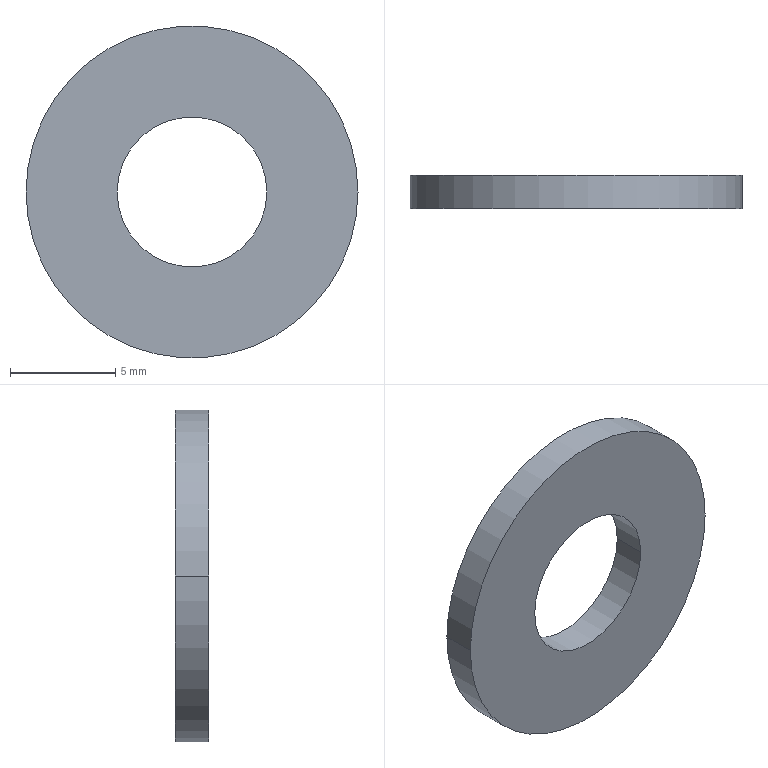Part | NX | features BREP 1 | 1 solid | 6 faces | box 15.748 x 1.575 x 15.748 mm | volume 244.177 mm3 | cylinder 4 | plane 2 | commonest cylinder face diameters 7.112 x2 15.748 x2
STEP:
#1=CARTESIAN_POINT('',(-7.874,0.,0.));
#2=VERTEX_POINT('',#1);
#3=CARTESIAN_POINT('',(7.874,0.,0.));
#4=VERTEX_POINT('',#3);
#5=CARTESIAN_POINT('',(0.,0.,0.));
#6=DIRECTION('',(0.,1.,0.));
#7=DIRECTION('',(-1.,0.,0.));
#8=AXIS2_PLACEMENT_3D('',#5,#6,#7);
#9=CIRCLE('',#8,7.874);
#10=EDGE_CURVE('',#2,#4,#9,.T.);
#11=ORIENTED_EDGE('',*,*,#10,.F.);
#12=CARTESIAN_POINT('',(0.,0.,0.));
#13=DIRECTION('',(0.,1.,0.));
#14=DIRECTION('',(1.,0.,0.));
#15=AXIS2_PLACEMENT_3D('',#12,#13,#14);
#16=CIRCLE('',#15,7.874);
#17=EDGE_CURVE('',#4,#2,#16,.T.);
#18=ORIENTED_EDGE('',*,*,#17,.F.);
#19=EDGE_LOOP('',(#11,#18));
#20=FACE_BOUND('',#19,.T.);
#21=CARTESIAN_POINT('',(-3.556,0.,0.));
#22=VERTEX_POINT('',#21);
#23=CARTESIAN_POINT('',(3.556,0.,0.));
#24=VERTEX_POINT('',#23);
#25=CARTESIAN_POINT('',(0.,0.,0.));
#26=DIRECTION('',(0.,-1.,0.));
#27=DIRECTION('',(-1.,0.,0.));
#28=AXIS2_PLACEMENT_3D('',#25,#26,#27);
#29=CIRCLE('',#28,3.556);
#30=EDGE_CURVE('',#22,#24,#29,.T.);
#31=ORIENTED_EDGE('',*,*,#30,.F.);
#32=CARTESIAN_POINT('',(0.,0.,0.));
#33=DIRECTION('',(0.,-1.,0.));
#34=DIRECTION('',(1.,0.,0.));
#35=AXIS2_PLACEMENT_3D('',#32,#33,#34);
#36=CIRCLE('',#35,3.556);
#37=EDGE_CURVE('',#24,#22,#36,.T.);
#38=ORIENTED_EDGE('',*,*,#37,.F.);
#39=EDGE_LOOP('',(#31,#38));
#40=FACE_BOUND('',#39,.T.);
#41=CARTESIAN_POINT('',(0.,0.,0.));
#42=DIRECTION('',(0.,1.,0.));
#43=DIRECTION('',(1.,0.,0.));
#44=AXIS2_PLACEMENT_3D('',#41,#42,#43);
#45=PLANE('',#44);
#46=ADVANCED_FACE('',(#20,#40),#45,.F.);
#47=CARTESIAN_POINT('',(-7.874,1.575,0.));
#48=VERTEX_POINT('',#47);
#49=CARTESIAN_POINT('',(-7.874,0.,0.));
#50=DIRECTION('',(0.,1.,0.));
#51=VECTOR('',#50,1000.);
#52=LINE('',#49,#51);
#53=EDGE_CURVE('',#2,#48,#52,.T.);
#54=ORIENTED_EDGE('',*,*,#53,.T.);
#55=CARTESIAN_POINT('',(7.874,1.575,0.));
#56=VERTEX_POINT('',#55);
#57=CARTESIAN_POINT('',(0.,1.575,0.));
#58=DIRECTION('',(0.,1.,0.));
#59=DIRECTION('',(1.,0.,0.));
#60=AXIS2_PLACEMENT_3D('',#57,#58,#59);
#61=CIRCLE('',#60,7.874);
#62=EDGE_CURVE('',#56,#48,#61,.T.);
#63=ORIENTED_EDGE('',*,*,#62,.F.);
#64=CARTESIAN_POINT('',(7.874,0.,0.));
#65=DIRECTION('',(0.,1.,0.));
#66=VECTOR('',#65,1000.);
#67=LINE('',#64,#66);
#68=EDGE_CURVE('',#4,#56,#67,.T.);
#69=ORIENTED_EDGE('',*,*,#68,.F.);
#70=ORIENTED_EDGE('',*,*,#17,.T.);
#71=EDGE_LOOP('',(#54,#63,#69,#70));
#72=FACE_BOUND('',#71,.T.);
#73=CARTESIAN_POINT('',(0.,0.,0.));
#74=DIRECTION('',(0.,1.,0.));
#75=DIRECTION('',(1.,0.,0.));
#76=AXIS2_PLACEMENT_3D('',#73,#74,#75);
#77=CYLINDRICAL_SURFACE('',#76,7.874);
#78=ADVANCED_FACE('',(#72),#77,.T.);
#79=ORIENTED_EDGE('',*,*,#68,.T.);
#80=CARTESIAN_POINT('',(0.,1.575,0.));
#81=DIRECTION('',(0.,1.,0.));
#82=DIRECTION('',(-1.,0.,0.));
#83=AXIS2_PLACEMENT_3D('',#80,#81,#82);
#84=CIRCLE('',#83,7.874);
#85=EDGE_CURVE('',#48,#56,#84,.T.);
#86=ORIENTED_EDGE('',*,*,#85,.F.);
#87=ORIENTED_EDGE('',*,*,#53,.F.);
#88=ORIENTED_EDGE('',*,*,#10,.T.);
#89=EDGE_LOOP('',(#79,#86,#87,#88));
#90=FACE_BOUND('',#89,.T.);
#91=CARTESIAN_POINT('',(0.,0.,0.));
#92=DIRECTION('',(0.,1.,0.));
#93=DIRECTION('',(1.,0.,0.));
#94=AXIS2_PLACEMENT_3D('',#91,#92,#93);
#95=CYLINDRICAL_SURFACE('',#94,7.874);
#96=ADVANCED_FACE('',(#90),#95,.T.);
#97=ORIENTED_EDGE('',*,*,#85,.T.);
#98=ORIENTED_EDGE('',*,*,#62,.T.);
#99=EDGE_LOOP('',(#97,#98));
#100=FACE_BOUND('',#99,.T.);
#101=CARTESIAN_POINT('',(-3.556,1.575,0.));
#102=VERTEX_POINT('',#101);
#103=CARTESIAN_POINT('',(3.556,1.575,0.));
#104=VERTEX_POINT('',#103);
#105=CARTESIAN_POINT('',(0.,1.575,0.));
#106=DIRECTION('',(0.,-1.,0.));
#107=DIRECTION('',(-1.,0.,0.));
#108=AXIS2_PLACEMENT_3D('',#105,#106,#107);
#109=CIRCLE('',#108,3.556);
#110=EDGE_CURVE('',#102,#104,#109,.T.);
#111=ORIENTED_EDGE('',*,*,#110,.T.);
#112=CARTESIAN_POINT('',(0.,1.575,0.));
#113=DIRECTION('',(0.,-1.,0.));
#114=DIRECTION('',(1.,0.,0.));
#115=AXIS2_PLACEMENT_3D('',#112,#113,#114);
#116=CIRCLE('',#115,3.556);
#117=EDGE_CURVE('',#104,#102,#116,.T.);
#118=ORIENTED_EDGE('',*,*,#117,.T.);
#119=EDGE_LOOP('',(#111,#118));
#120=FACE_BOUND('',#119,.T.);
#121=CARTESIAN_POINT('',(0.,1.575,0.));
#122=DIRECTION('',(0.,1.,0.));
#123=DIRECTION('',(1.,0.,0.));
#124=AXIS2_PLACEMENT_3D('',#121,#122,#123);
#125=PLANE('',#124);
#126=ADVANCED_FACE('',(#100,#120),#125,.T.);
#127=CARTESIAN_POINT('',(-3.556,0.,0.));
#128=DIRECTION('',(0.,1.,0.));
#129=VECTOR('',#128,1000.);
#130=LINE('',#127,#129);
#131=EDGE_CURVE('',#22,#102,#130,.T.);
#132=ORIENTED_EDGE('',*,*,#131,.T.);
#133=ORIENTED_EDGE('',*,*,#117,.F.);
#134=CARTESIAN_POINT('',(3.556,0.,0.));
#135=DIRECTION('',(0.,1.,0.));
#136=VECTOR('',#135,1000.);
#137=LINE('',#134,#136);
#138=EDGE_CURVE('',#24,#104,#137,.T.);
#139=ORIENTED_EDGE('',*,*,#138,.F.);
#140=ORIENTED_EDGE('',*,*,#37,.T.);
#141=EDGE_LOOP('',(#132,#133,#139,#140));
#142=FACE_BOUND('',#141,.T.);
#143=CARTESIAN_POINT('',(0.,0.,0.));
#144=DIRECTION('',(0.,1.,0.));
#145=DIRECTION('',(1.,0.,0.));
#146=AXIS2_PLACEMENT_3D('',#143,#144,#145);
#147=CYLINDRICAL_SURFACE('',#146,3.556);
#148=ADVANCED_FACE('',(#142),#147,.F.);
#149=ORIENTED_EDGE('',*,*,#138,.T.);
#150=ORIENTED_EDGE('',*,*,#110,.F.);
#151=ORIENTED_EDGE('',*,*,#131,.F.);
#152=ORIENTED_EDGE('',*,*,#30,.T.);
#153=EDGE_LOOP('',(#149,#150,#151,#152));
#154=FACE_BOUND('',#153,.T.);
#155=CARTESIAN_POINT('',(0.,0.,0.));
#156=DIRECTION('',(0.,1.,0.));
#157=DIRECTION('',(1.,0.,0.));
#158=AXIS2_PLACEMENT_3D('',#155,#156,#157);
#159=CYLINDRICAL_SURFACE('',#158,3.556);
#160=ADVANCED_FACE('',(#154),#159,.F.);
#161=CLOSED_SHELL('',(#46,#78,#96,#126,#148,#160));
#162=MANIFOLD_SOLID_BREP('',#161);
#163=(LENGTH_UNIT()NAMED_UNIT(*)SI_UNIT(.MILLI.,.METRE.));
#164=UNCERTAINTY_MEASURE_WITH_UNIT(LENGTH_MEASURE(0.00001),#163,'','');
#165=(NAMED_UNIT(*)PLANE_ANGLE_UNIT()SI_UNIT($,.RADIAN.));
#166=(NAMED_UNIT(*)SI_UNIT($,.STERADIAN.)SOLID_ANGLE_UNIT());
#167=(GEOMETRIC_REPRESENTATION_CONTEXT(3)GLOBAL_UNCERTAINTY_ASSIGNED_CONTEXT((#164))GLOBAL_UNIT_ASSIGNED_CONTEXT((#163,#165,#166))REPRESENTATION_CONTEXT('',''));
#168=ADVANCED_BREP_SHAPE_REPRESENTATION('',(#162),#167);